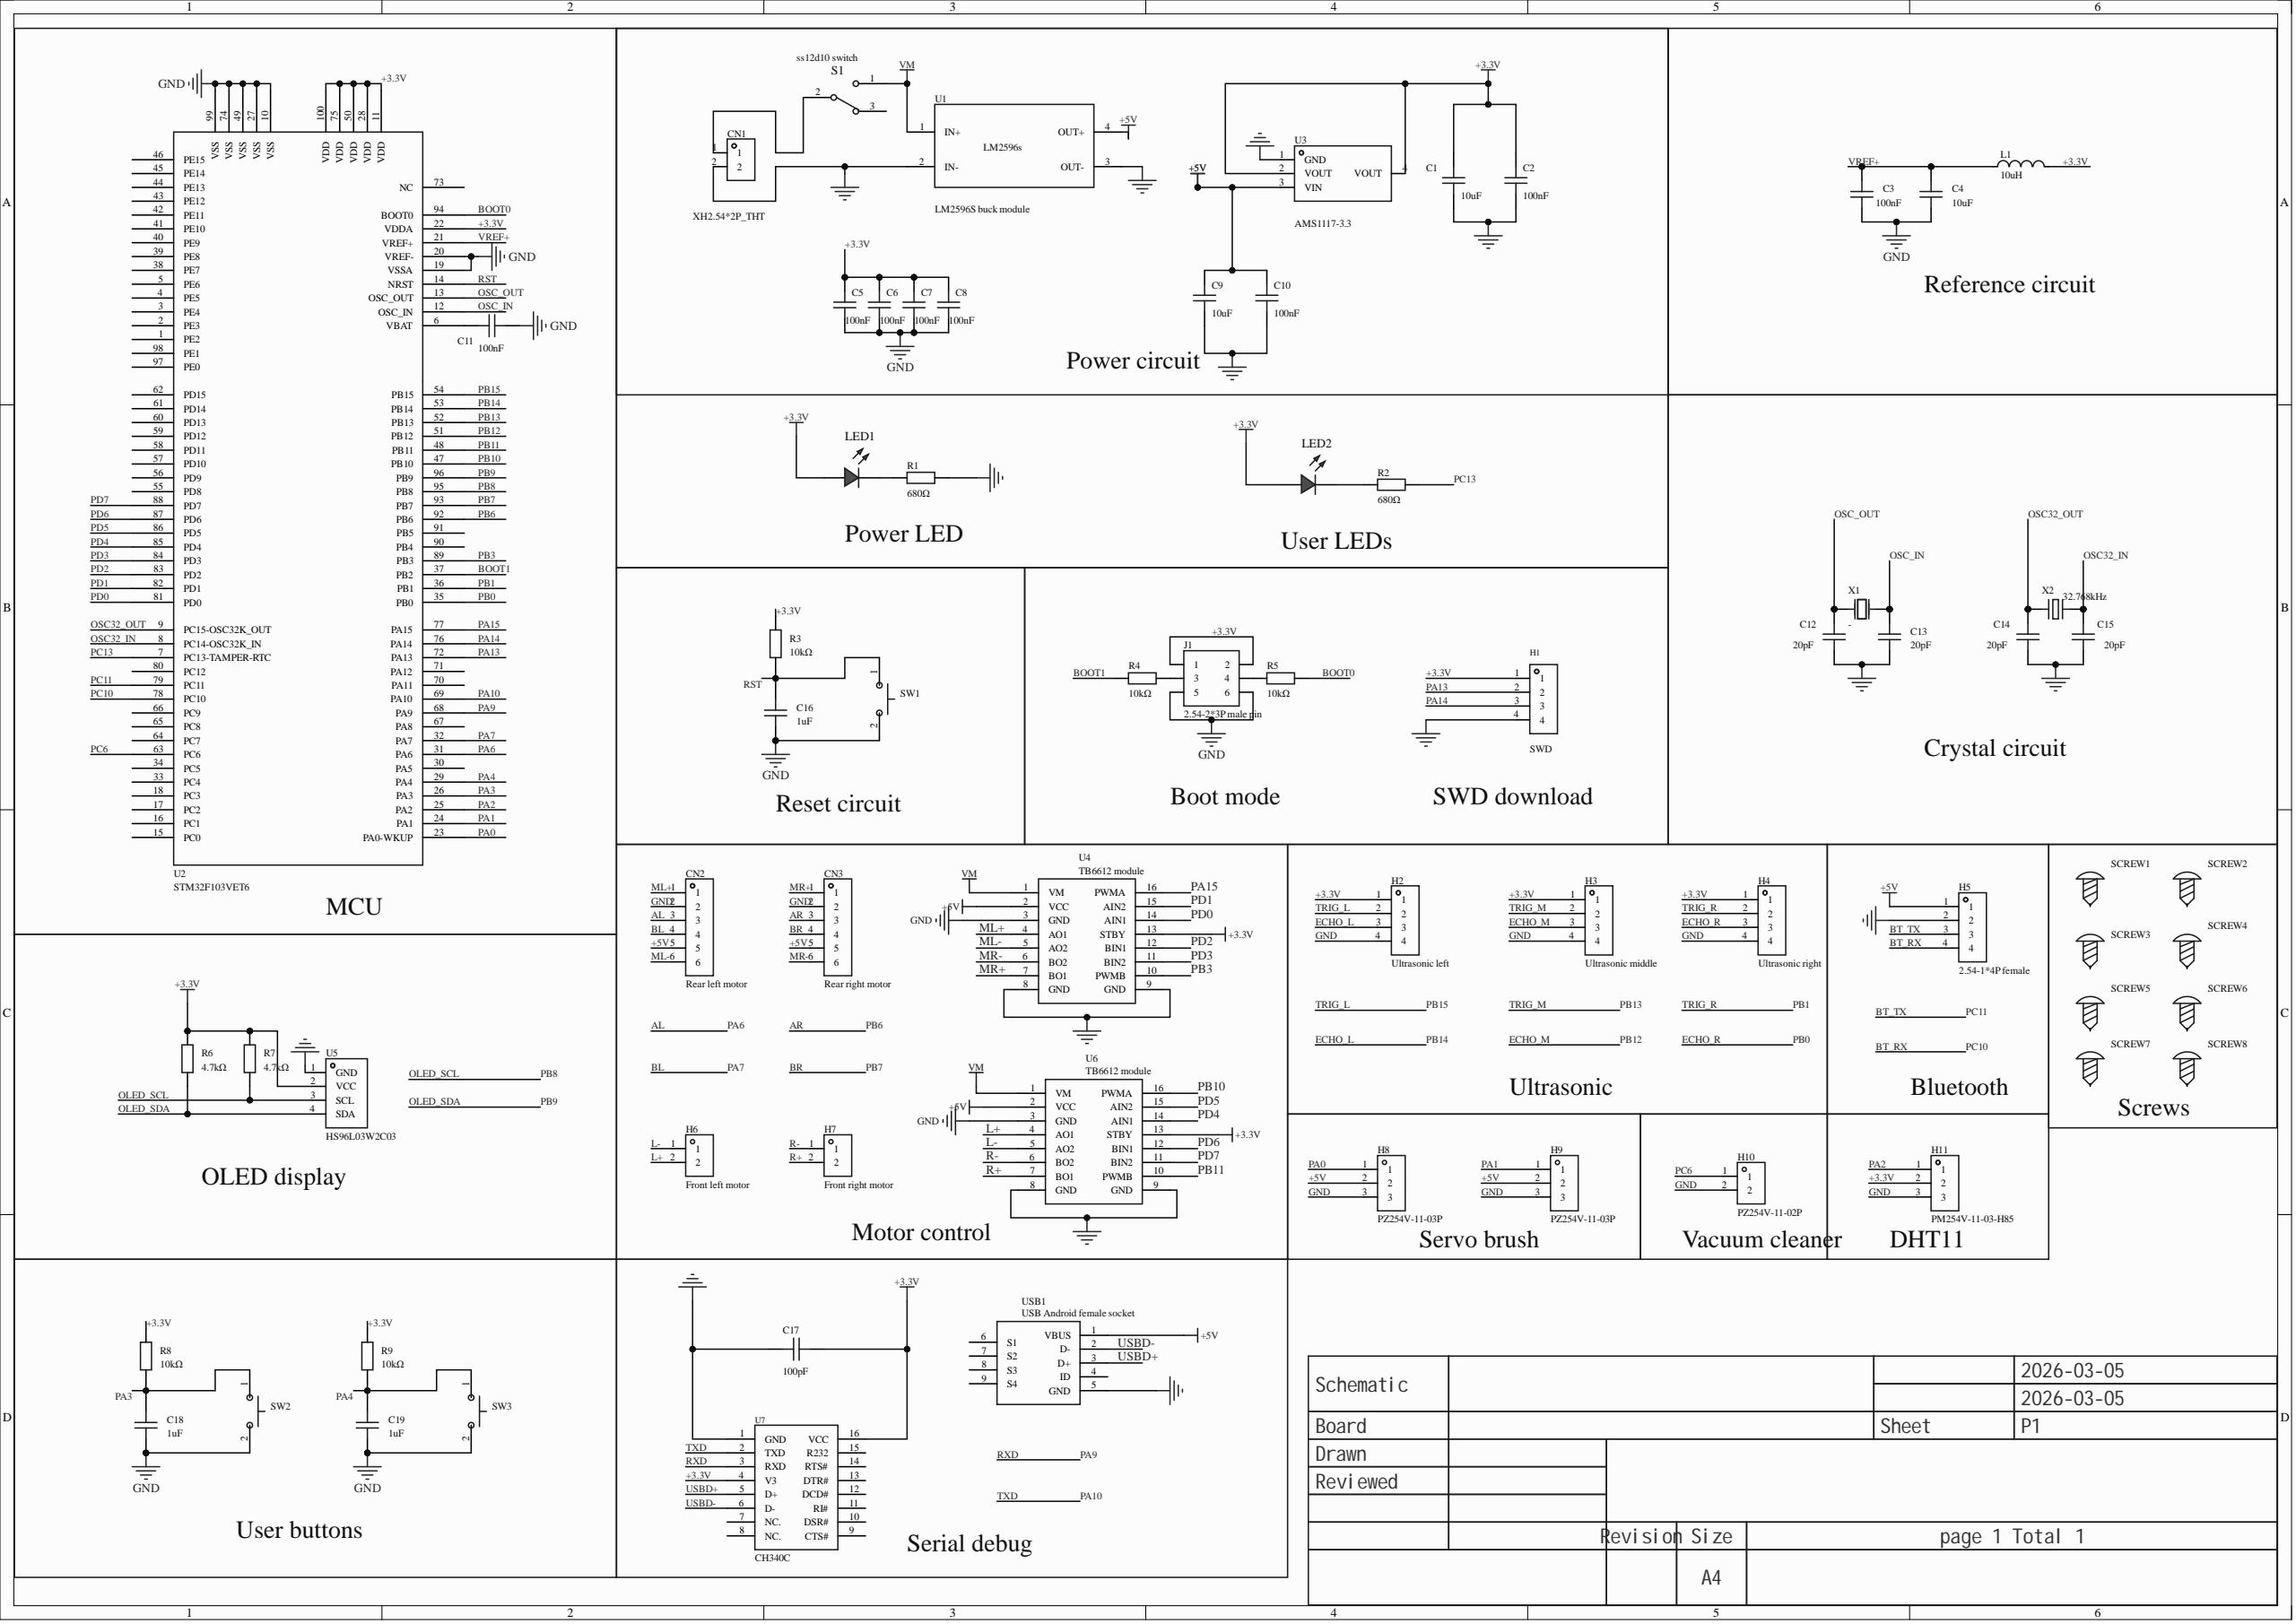Circuit board | Altium Designer | 68 parts | 65 nets
Bill of materials:
Comment,Description,Designator,Footprint,LibRef,Quantity
"10uF","Capacitance:10uF;Tolerance:±10%;Rated voltage:50V;Dielectric (temp. coeff.):X5R;","C1, C9","C0805","GRM21BR61H106KE43L","2"
"100nF","Capacitance:100nF;Tolerance:±10%;Rated voltage:50V;Dielectric (temp. coeff.):X7R;","C2, C10","C0805","CL21B104KBCNNNC","2"
"100nF","Capacitance:100nF;Tolerance:±10%;Rated voltage:50V;Dielectric (temp. coeff.):X7R;","C3, C5, C6, C7, C8, C11","C0603","CC0603KRX7R9BB104","6"
"10uF","Capacitance:10uF;Tolerance:±10%;Rated voltage:10V;Dielectric:X5R;","C4","C0603","CL10A106KP8NNNC","1"
"20pF","Capacitance:20pF;Tolerance:±5%;Rated voltage:50V;Dielectric:C0G;","C12, C13, C14, C15","C0805","CL21C200JBANNNC","4"
"1uF","Capacitance:1uF;Tolerance:±10%;Rated voltage:50V;Dielectric:X5R;","C16, C18, C19","C0603","CL10A105KB8NNNC","3"
"100pF","Capacitance:100pF;Tolerance:±5%;Rated voltage:50V;Dielectric:C0G;","C17","C0805","CL21C101JBANNNC","1"
"XH2.54*2P_THT","","CN1","CONN-TH_2P-P2.50-XH2.54-2P","XH2.54*2P_直插","1"
"Rear left motor","","CN2","CONN-TH_XH2.54-6P","XH2.54*6P_直插","1"
"Rear right motor","","CN3","CONN-TH_XH2.54-6P","XH2.54*6P_直插","1"
"SWD","","H1","HDR-TH_4P-P2.54-V-M","KH-2.54PH180-1X4P-L11.5","1"
"Ultrasonic left","","H2","HDR-TH_4P-P2.54-V-M","PZ254V-11-04P","1"
"Ultrasonic middle","","H3","HDR-TH_4P-P2.54-V-M","PZ254V-11-04P","1"
"Ultrasonic right","","H4","HDR-TH_4P-P2.54-V-M","PZ254V-11-04P","1"
"2.54-1*4P female","","H5","HDR-TH_4P-P2.54-V-F","2.54-1*4P母","1"
"Front left motor","","H6","HDR-TH_2P-P2.54-V-M","PZ254V-11-02P","1"
"Front right motor","","H7","HDR-TH_2P-P2.54-V-M","PZ254V-11-02P","1"
"PZ254V-11-03P","","H8, H9","HDR-TH_3P-P2.54-V-M","PZ254V-11-03P","2"
"PZ254V-11-02P","","H10","HDR-TH_2P-P2.54-V-M","PZ254V-11-02P","1"
"PM254V-11-03-H85","Socket structure:1x3P;Pitch:2.54mm;Row spacing:-;Mounting type:Through-hole;Rows:Single;Total hole count:3P;Plastic height:-;Contact material:Brass;Contact plating:-;","H11","HDR-TH_3P-P2.54-V-F","PM254V-11-03-H85","1"
"2.54-2*3P male pin","","J1","HDR-TH_6P-P2.54-V-M-R2-C3-S2.54-1","2.54-2*3P针","1"
"10uH","Inductance:10uH;Tolerance:±10%;Rated current:3mA;Saturation current (Isat):-;DC resistance (DCR):1.85Ω;","L1","L0603","SDFL1608S100KTF","1"
"NCD0805R1","Emitted color:Red;","LED1, LED2","LED0805-RD_RED","NCD0805R1","2"
"680Ω","Resistor type:Thick-film resistor;Resistance:680Ω;Tolerance:±1%;Power:125mW;Max working voltage:150V;Temp. coeff.:±100ppm/?;","R1, R2","R0805","0805W8F6800T5E","2"
"10kΩ","Resistor type:Thick-film resistor;Resistance:10kΩ;Tolerance:±1%;Power:100mW;","R3, R4, R5, R8, R9","R0603","0603WAF1002T5E","5"
"4.7kΩ","Resistor type:Thick-film resistor;Resistance:4.7kΩ;Tolerance:±1%;Power:125mW;Max working voltage:150V;Temp. coeff.:±100ppm/?;","R6, R7","R0805","0805W8F4701T5E","2"
"ss12d10 switch","","S1","SS12D10","SS12D10","1"
"","","SCREW1, SCREW2, SCREW3, SCREW4","M3螺丝","M3螺丝","4"
"","","SCREW5, SCREW6, SCREW7, SCREW8","M2螺丝","M2螺丝","4"
"1TS002C-2300-4300-CT","","SW1, SW2, SW3","SW-SMD_L6.0-W3.5-LS8.0-EH","1TS002C-2300-4300-CT","3"
"LM2596S buck module","","U1","LM2596S","LM2596S","1"
"STM32F103VET6","CPU core:ARM-M3;Max CPU frequency:72MHz;Application field:-;","U2","LQFP-100_L14.0-W14.0-P0.50-LS16.0-BL","STM32F103VET6","1"
"AMS1117-3.3","Output type:Fixed;Output polarity:Positive;Max input voltage:-;Output voltage:3.3V;Output current:1A;Power supply rejection ratio (PSRR):72dB@(120Hz);","U3","SOT-223-3_L6.5-W3.4-P2.30-LS7.0-BR","AMS1117-3.3_C6186","1"
"TB6612 module","","U4, U6","TB6612-2X8","TB6612模块","2"
"HS96L03W2C03","Main controller:SSD1315;Interface type:I2C;Size (inch):0.96;Pixel resolution:128x64;","U5","OLED-TH_L27.8-W27.2-P2.54_C9900033791","HS96L03W2C03","1"
"CH340C","Application function:Transceiver;Interface protocol:USB 2.0;Data rate:2Mbps;","U7","SOP-16_L10.0-W3.9-P1.27-LS6.0-BL","CH340C","1"
"USB Android female socket","","USB1","MICRO-USB-SMD_MICRO-USB-A8","USB安卓母座","1"
"-","Frequency:-;Load capacitance:-;","X1","HC-49US_L11.5-W4.5-P4.88","9B08000368","1"
"32.768kHz","Frequency:32.768kHz;Frequency tolerance:±20ppm;Load capacitance:12.5pF;","X2","OSC-SMD_L3.2-W1.5","X321532768KGD2SI","1"
Netlist (Protel format):
[
C1
C0805
10uF



]
[
C2
C0805
100nF



]
[
C3
C0603
100nF



]
[
C4
C0603
10uF



]
[
C5
C0603
100nF



]
[
C6
C0603
100nF



]
[
C7
C0603
100nF



]
[
C8
C0603
100nF



]
[
C9
C0805
10uF



]
[
C10
C0805
100nF



]
[
C11
C0603
100nF



]
[
C12
C0805
20pF



]
[
C13
C0805
20pF



]
[
C14
C0805
20pF



]
[
C15
C0805
20pF



]
[
C16
C0603
1uF



]
[
C17
C0805
100pF



]
[
C18
C0603
1uF



]
[
C19
C0603
1uF



]
[
CN1
CONN-TH_2P-P2.50-XH2.54-2P
XH2.54*2P_THT



]
[
CN2
CONN-TH_XH2.54-6P
Rear left motor



]
[
CN3
CONN-TH_XH2.54-6P
Rear right motor



]
[
H1
HDR-TH_4P-P2.54-V-M
SWD



]
[
H2
HDR-TH_4P-P2.54-V-M
Ultrasonic left



]
[
H3
HDR-TH_4P-P2.54-V-M
Ultrasonic middle



]
[
H4
HDR-TH_4P-P2.54-V-M
Ultrasonic right



]
[
H5
HDR-TH_4P-P2.54-V-F
2.54-1*4P female



]
[
H6
HDR-TH_2P-P2.54-V-M
Front left motor



]
[
H7
HDR-TH_2P-P2.54-V-M
Front right motor



]
[
H8
HDR-TH_3P-P2.54-V-M
PZ254V-11-03P



]
[
H9
HDR-TH_3P-P2.54-V-M
PZ254V-11-03P



]
[
H10
HDR-TH_2P-P2.54-V-M
PZ254V-11-02P



]
[
H11
HDR-TH_3P-P2.54-V-F
PM254V-11-03-H85



]
[
J1
HDR-TH_6P-P2.54-V-M-R2-C3-S2.54-1
2.54-2*3P male pin



]
[
L1
L0603
10uH



]
[
LED1
LED0805-RD_RED
NCD0805R1



]
[
LED2
LED0805-RD_RED
NCD0805R1



]
[
R1
R0805
680Ω



]
[
R2
R0805
680Ω



]
[
R3
R0603
10kΩ



]
[
R4
R0603
10kΩ



]
[
R5
R0603
10kΩ



]
[
R6
R0805
4.7kΩ



]
[
R7
R0805
4.7kΩ



]
[
R8
R0603
10kΩ



]
[
R9
R0603
10kΩ



]
[
S1
SS12D10
ss12d10 switch



]
[
SCREW1
M3螺丝




]
[
SCREW2
M3螺丝




]
[
SCREW3
M3螺丝




]
[
SCREW4
M3螺丝




]
[
SCREW5
M2螺丝




]
[
SCREW6
M2螺丝




]
[
SCREW7
M2螺丝




]
[
SCREW8
M2螺丝




]
[
SW1
SW-SMD_L6.0-W3.5-LS8.0-EH
1TS002C-2300-4300-CT



]
[
SW2
SW-SMD_L6.0-W3.5-LS8.0-EH
1TS002C-2300-4300-CT



]
[
SW3
SW-SMD_L6.0-W3.5-LS8.0-EH
1TS002C-2300-4300-CT



]
[
U1
LM2596S
LM2596S buck module



]
[
U2
LQFP-100_L14.0-W14.0-P0.50-LS16.0-BL
STM32F103VET6



]
[
U3
SOT-223-3_L6.5-W3.4-P2.30-LS7.0-BR
AMS1117-3.3



]
[
U4
TB6612-2X8
TB6612 module



]
[
U5
OLED-TH_L27.8-W27.2-P2.54_C9900033791
HS96L03W2C03



]
[
U6
TB6612-2X8
TB6612 module



]
[
U7
SOP-16_L10.0-W3.9-P1.27-LS6.0-BL
CH340C



]
[
USB1
MICRO-USB-SMD_MICRO-USB-A8
USB Android female socket



]
[
X1
HC-49US_L11.5-W4.5-P4.88
-



]
[
X2
OSC-SMD_L3.2-W1.5
32.768kHz



]
(
VREF+
C3-2
C4-2
L1-1
U2-21
)
(
VM
S1-1
U1-1
U4-1
U6-1
)
(
USBD-
U7-6
USB1-2
)
(
USBD+
U7-5
USB1-3
)
(
RST
C16-2
R3-1
SW1-1
U2-14
)
(
R-
H7-1
U6-6
)
(
R+
H7-2
U6-7
)
(
PD7
U2-88
U6-11
)
(
PD6
U2-87
U6-12
)
(
PD5
U2-86
U6-15
)
(
PD4
U2-85
U6-14
)
(
PD3
U2-84
U4-11
)
(
PD2
U2-83
U4-12
)
(
PD1
U2-82
U4-15
)
(
PD0
U2-81
U4-14
)
(
PC13
R2-2
U2-7
)
(
PC6
H10-1
U2-63
)
(
PB15
H2-2
U2-54
)
(
PB13
H3-2
U2-52
)
(
PB11
U2-48
U6-10
)
(
PB10
U2-47
U6-16
)
(
PB3
U2-89
U4-10
)
(
PB1
H4-2
U2-36
)
(
PA15
U2-77
U4-16
)
(
PA14
H1-3
U2-76
)
(
PA13
H1-2
U2-72
)
(
PA10
U2-69
U7-2
)
(
PA9
U2-68
U7-3
)
(
PA4
C19-2
R9-1
SW3-1
U2-29
)
(
PA3
C18-2
R8-1
SW2-1
U2-26
)
(
PA2
H11-1
U2-25
)
(
PA1
H9-1
U2-24
)
(
PA0
H8-1
U2-23
)
(
OSC_OUT
C12-2
U2-13
X1-1
)
(
OSC_IN
C13-2
U2-12
X1-2
)
(
OSC32_OUT
C14-2
U2-9
X2-1
)
(
OSC32_IN
C15-2
U2-8
X2-2
)
(
OLED_SDA
R6-2
U2-96
U5-4
)
(
OLED_SCL
R7-2
U2-95
U5-3
)
(
NetLED2_1
LED2-1
R2-1
)
(
NetLED1_1
LED1-1
R1-1
)
(
NetJ1_4
J1-4
R5-1
)
(
NetJ1_3
J1-3
R4-2
)
(
NetCN1_1
CN1-1
S1-2
)
(
NetC11_1
C11-1
U2-6
)
(
MR-
CN3-6
U4-6
)
(
MR+
CN3-1
U4-7
)
(
ML-
CN2-6
U4-5
)
(
ML+
CN2-1
U4-4
)
(
L-
H6-1
U6-5
)
(
L+
H6-2
U6-4
)
(
GND
C1-1
C2-1
C3-1
C4-1
C5-2
C6-2
C7-2
C8-2
C9-1
C10-1
C11-2
C12-1
C13-1
C14-1
C15-1
C16-1
C17-1
C18-1
C19-1
CN1-2
CN2-2
CN3-2
H1-4
H2-4
H3-4
H4-4
H5-2
H8-3
H9-3
H10-2
H11-3
J1-5
J1-6
R1-2
SW1-2
SW2-2
SW3-2
U1-2
U1-3
U2-10
U2-19
U2-20
U2-27
U2-49
U2-74
U2-99
U3-1
U4-3
U4-8
U4-9
U5-1
U6-3
U6-8
U6-9
U7-1
USB1-5
)
(
ECHO_R
H4-3
U2-35
)
(
ECHO_M
H3-3
U2-51
)
(
ECHO_L
H2-3
U2-53
)
(
BT_TX
H5-3
U2-79
)
(
BT_RX
H5-4
U2-78
)
(
BR
CN3-4
U2-93
)
(
BOOT1
R4-1
U2-37
)
(
BOOT0
R5-2
U2-94
)
(
BL
CN2-4
U2-32
)
(
AR
CN3-3
U2-92
)
(
AL
CN2-3
U2-31
)
(
+5V
C9-2
C10-2
CN2-5
CN3-5
H5-1
H8-2
H9-2
U1-4
U3-3
U4-2
U6-2
USB1-1
)
(
+3.3V
C1-2
C2-2
C5-1
C6-1
C7-1
C8-1
C17-2
H1-1
H2-1
H3-1
H4-1
H11-2
J1-1
J1-2
L1-2
LED1-2
LED2-2
R3-2
R6-1
R7-1
R8-2
R9-2
U2-11
U2-22
U2-28
U2-50
U2-75
U2-100
U3-2
U3-4
U4-13
U5-2
U6-13
U7-4
U7-16
)